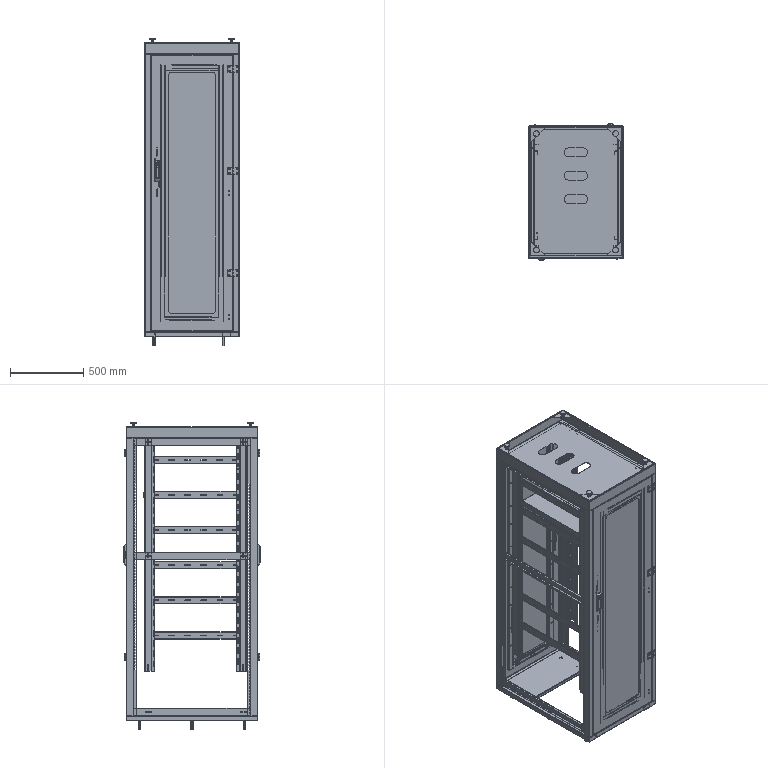Part | SolidWorks | features ReferencePattern 2, LocalLPattern 1 | 91 solids | 7729 faces | volume 20009952 mm3 | plane 5196 | cylinder 2337 | spline 116 | cone 80 | commonest cylinder face diameters 6 x689 5 x602 7 x314 12 x200 2 x183 10 x110